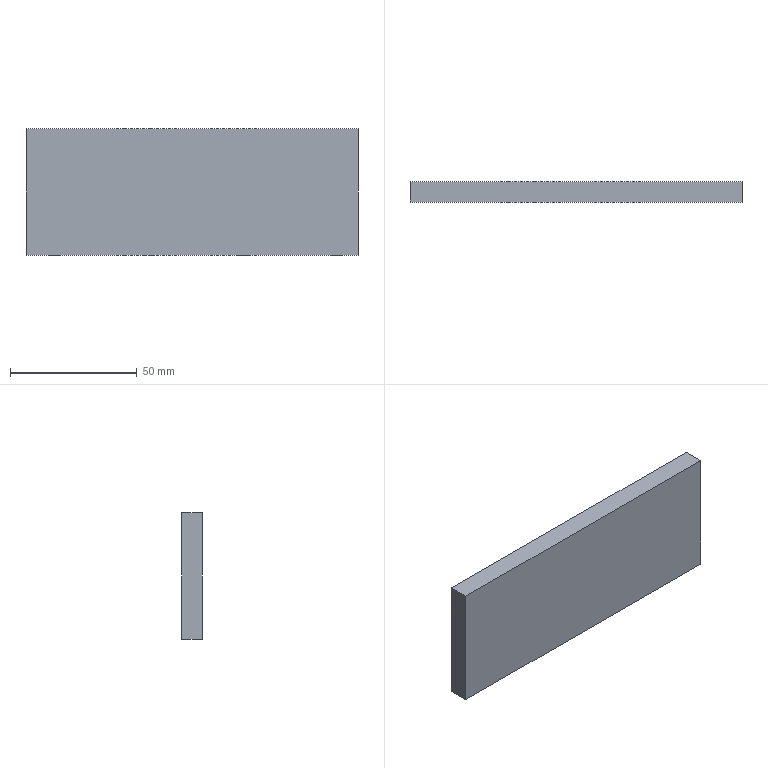Part | SolidWorks | features Extrusion 1, ICE 1 | 1 solid | 18 faces | box 131 x 8 x 50 mm | volume 51646 mm3 | plane 10 | cylinder 8 | commonest cylinder face diameters 4 x8
STEP:
#1=CARTESIAN_POINT('',(124.391,4.,15.));
#2=VERTEX_POINT('',#1);
#3=CARTESIAN_POINT('',(120.391,4.,15.));
#4=VERTEX_POINT('',#3);
#5=CARTESIAN_POINT('',(122.391,4.,15.));
#6=DIRECTION('',(0.,0.,-1.));
#7=DIRECTION('',(-1.,0.,0.));
#8=AXIS2_PLACEMENT_3D('',#5,#6,#7);
#9=CIRCLE('',#8,2.);
#10=EDGE_CURVE('',#2,#4,#9,.T.);
#11=ORIENTED_EDGE('',*,*,#10,.F.);
#12=CARTESIAN_POINT('',(124.391,4.,0.));
#13=VERTEX_POINT('',#12);
#14=CARTESIAN_POINT('',(124.391,4.,15.));
#15=DIRECTION('',(0.,0.,-1.));
#16=VECTOR('',#15,1000.);
#17=LINE('',#14,#16);
#18=EDGE_CURVE('',#2,#13,#17,.T.);
#19=ORIENTED_EDGE('',*,*,#18,.T.);
#20=CARTESIAN_POINT('',(120.391,4.,0.));
#21=VERTEX_POINT('',#20);
#22=CARTESIAN_POINT('',(122.391,4.,0.));
#23=DIRECTION('',(0.,0.,-1.));
#24=DIRECTION('',(-1.,0.,0.));
#25=AXIS2_PLACEMENT_3D('',#22,#23,#24);
#26=CIRCLE('',#25,2.);
#27=EDGE_CURVE('',#13,#21,#26,.T.);
#28=ORIENTED_EDGE('',*,*,#27,.T.);
#29=CARTESIAN_POINT('',(120.391,4.,15.));
#30=DIRECTION('',(0.,0.,-1.));
#31=VECTOR('',#30,1000.);
#32=LINE('',#29,#31);
#33=EDGE_CURVE('',#4,#21,#32,.T.);
#34=ORIENTED_EDGE('',*,*,#33,.F.);
#35=EDGE_LOOP('',(#11,#19,#28,#34));
#36=FACE_OUTER_BOUND('',#35,.T.);
#37=CARTESIAN_POINT('',(122.391,4.,15.));
#38=DIRECTION('',(0.,0.,-1.));
#39=DIRECTION('',(-1.,0.,0.));
#40=AXIS2_PLACEMENT_3D('',#37,#38,#39);
#41=CYLINDRICAL_SURFACE('',#40,2.);
#42=ADVANCED_FACE('',(#36),#41,.F.);
#43=CARTESIAN_POINT('',(87.391,4.,15.));
#44=VERTEX_POINT('',#43);
#45=CARTESIAN_POINT('',(83.391,4.,15.));
#46=VERTEX_POINT('',#45);
#47=CARTESIAN_POINT('',(85.391,4.,15.));
#48=DIRECTION('',(0.,0.,-1.));
#49=DIRECTION('',(-1.,0.,0.));
#50=AXIS2_PLACEMENT_3D('',#47,#48,#49);
#51=CIRCLE('',#50,2.);
#52=EDGE_CURVE('',#44,#46,#51,.T.);
#53=ORIENTED_EDGE('',*,*,#52,.F.);
#54=CARTESIAN_POINT('',(87.391,4.,0.));
#55=VERTEX_POINT('',#54);
#56=CARTESIAN_POINT('',(87.391,4.,15.));
#57=DIRECTION('',(0.,0.,-1.));
#58=VECTOR('',#57,1000.);
#59=LINE('',#56,#58);
#60=EDGE_CURVE('',#44,#55,#59,.T.);
#61=ORIENTED_EDGE('',*,*,#60,.T.);
#62=CARTESIAN_POINT('',(83.391,4.,0.));
#63=VERTEX_POINT('',#62);
#64=CARTESIAN_POINT('',(85.391,4.,0.));
#65=DIRECTION('',(0.,0.,-1.));
#66=DIRECTION('',(-1.,0.,0.));
#67=AXIS2_PLACEMENT_3D('',#64,#65,#66);
#68=CIRCLE('',#67,2.);
#69=EDGE_CURVE('',#55,#63,#68,.T.);
#70=ORIENTED_EDGE('',*,*,#69,.T.);
#71=CARTESIAN_POINT('',(83.391,4.,15.));
#72=DIRECTION('',(0.,0.,-1.));
#73=VECTOR('',#72,1000.);
#74=LINE('',#71,#73);
#75=EDGE_CURVE('',#46,#63,#74,.T.);
#76=ORIENTED_EDGE('',*,*,#75,.F.);
#77=EDGE_LOOP('',(#53,#61,#70,#76));
#78=FACE_OUTER_BOUND('',#77,.T.);
#79=CARTESIAN_POINT('',(85.391,4.,15.));
#80=DIRECTION('',(0.,0.,-1.));
#81=DIRECTION('',(-1.,0.,0.));
#82=AXIS2_PLACEMENT_3D('',#79,#80,#81);
#83=CYLINDRICAL_SURFACE('',#82,2.);
#84=ADVANCED_FACE('',(#78),#83,.F.);
#85=CARTESIAN_POINT('',(50.391,4.,15.));
#86=VERTEX_POINT('',#85);
#87=CARTESIAN_POINT('',(46.391,4.,15.));
#88=VERTEX_POINT('',#87);
#89=CARTESIAN_POINT('',(48.391,4.,15.));
#90=DIRECTION('',(0.,0.,-1.));
#91=DIRECTION('',(-1.,0.,0.));
#92=AXIS2_PLACEMENT_3D('',#89,#90,#91);
#93=CIRCLE('',#92,2.);
#94=EDGE_CURVE('',#86,#88,#93,.T.);
#95=ORIENTED_EDGE('',*,*,#94,.F.);
#96=CARTESIAN_POINT('',(50.391,4.,0.));
#97=VERTEX_POINT('',#96);
#98=CARTESIAN_POINT('',(50.391,4.,15.));
#99=DIRECTION('',(0.,0.,-1.));
#100=VECTOR('',#99,1000.);
#101=LINE('',#98,#100);
#102=EDGE_CURVE('',#86,#97,#101,.T.);
#103=ORIENTED_EDGE('',*,*,#102,.T.);
#104=CARTESIAN_POINT('',(46.391,4.,0.));
#105=VERTEX_POINT('',#104);
#106=CARTESIAN_POINT('',(48.391,4.,0.));
#107=DIRECTION('',(0.,0.,-1.));
#108=DIRECTION('',(-1.,0.,0.));
#109=AXIS2_PLACEMENT_3D('',#106,#107,#108);
#110=CIRCLE('',#109,2.);
#111=EDGE_CURVE('',#97,#105,#110,.T.);
#112=ORIENTED_EDGE('',*,*,#111,.T.);
#113=CARTESIAN_POINT('',(46.391,4.,15.));
#114=DIRECTION('',(0.,0.,-1.));
#115=VECTOR('',#114,1000.);
#116=LINE('',#113,#115);
#117=EDGE_CURVE('',#88,#105,#116,.T.);
#118=ORIENTED_EDGE('',*,*,#117,.F.);
#119=EDGE_LOOP('',(#95,#103,#112,#118));
#120=FACE_OUTER_BOUND('',#119,.T.);
#121=CARTESIAN_POINT('',(48.391,4.,15.));
#122=DIRECTION('',(0.,0.,-1.));
#123=DIRECTION('',(-1.,0.,0.));
#124=AXIS2_PLACEMENT_3D('',#121,#122,#123);
#125=CYLINDRICAL_SURFACE('',#124,2.);
#126=ADVANCED_FACE('',(#120),#125,.F.);
#127=CARTESIAN_POINT('',(13.391,4.,15.));
#128=VERTEX_POINT('',#127);
#129=CARTESIAN_POINT('',(9.391,4.,15.));
#130=VERTEX_POINT('',#129);
#131=CARTESIAN_POINT('',(11.391,4.,15.));
#132=DIRECTION('',(0.,0.,-1.));
#133=DIRECTION('',(-1.,0.,0.));
#134=AXIS2_PLACEMENT_3D('',#131,#132,#133);
#135=CIRCLE('',#134,2.);
#136=EDGE_CURVE('',#128,#130,#135,.T.);
#137=ORIENTED_EDGE('',*,*,#136,.F.);
#138=CARTESIAN_POINT('',(13.391,4.,0.));
#139=VERTEX_POINT('',#138);
#140=CARTESIAN_POINT('',(13.391,4.,15.));
#141=DIRECTION('',(0.,0.,-1.));
#142=VECTOR('',#141,1000.);
#143=LINE('',#140,#142);
#144=EDGE_CURVE('',#128,#139,#143,.T.);
#145=ORIENTED_EDGE('',*,*,#144,.T.);
#146=CARTESIAN_POINT('',(9.391,4.,0.));
#147=VERTEX_POINT('',#146);
#148=CARTESIAN_POINT('',(11.391,4.,0.));
#149=DIRECTION('',(0.,0.,-1.));
#150=DIRECTION('',(-1.,0.,0.));
#151=AXIS2_PLACEMENT_3D('',#148,#149,#150);
#152=CIRCLE('',#151,2.);
#153=EDGE_CURVE('',#139,#147,#152,.T.);
#154=ORIENTED_EDGE('',*,*,#153,.T.);
#155=CARTESIAN_POINT('',(9.391,4.,15.));
#156=DIRECTION('',(0.,0.,-1.));
#157=VECTOR('',#156,1000.);
#158=LINE('',#155,#157);
#159=EDGE_CURVE('',#130,#147,#158,.T.);
#160=ORIENTED_EDGE('',*,*,#159,.F.);
#161=EDGE_LOOP('',(#137,#145,#154,#160));
#162=FACE_OUTER_BOUND('',#161,.T.);
#163=CARTESIAN_POINT('',(11.391,4.,15.));
#164=DIRECTION('',(0.,0.,-1.));
#165=DIRECTION('',(-1.,0.,0.));
#166=AXIS2_PLACEMENT_3D('',#163,#164,#165);
#167=CYLINDRICAL_SURFACE('',#166,2.);
#168=ADVANCED_FACE('',(#162),#167,.F.);
#169=CARTESIAN_POINT('',(0.,8.,0.));
#170=VERTEX_POINT('',#169);
#171=CARTESIAN_POINT('',(0.,0.,0.));
#172=VERTEX_POINT('',#171);
#173=CARTESIAN_POINT('',(0.,0.,0.));
#174=DIRECTION('',(0.,-1.,0.));
#175=VECTOR('',#174,1000.);
#176=LINE('',#173,#175);
#177=EDGE_CURVE('',#170,#172,#176,.T.);
#178=ORIENTED_EDGE('',*,*,#177,.T.);
#179=CARTESIAN_POINT('',(0.,0.,50.));
#180=VERTEX_POINT('',#179);
#181=CARTESIAN_POINT('',(0.,0.,50.));
#182=DIRECTION('',(0.,0.,-1.));
#183=VECTOR('',#182,1000.);
#184=LINE('',#181,#183);
#185=EDGE_CURVE('',#180,#172,#184,.T.);
#186=ORIENTED_EDGE('',*,*,#185,.F.);
#187=CARTESIAN_POINT('',(0.,8.,50.));
#188=VERTEX_POINT('',#187);
#189=CARTESIAN_POINT('',(0.,0.,50.));
#190=DIRECTION('',(0.,-1.,0.));
#191=VECTOR('',#190,1000.);
#192=LINE('',#189,#191);
#193=EDGE_CURVE('',#188,#180,#192,.T.);
#194=ORIENTED_EDGE('',*,*,#193,.F.);
#195=CARTESIAN_POINT('',(0.,8.,50.));
#196=DIRECTION('',(0.,0.,-1.));
#197=VECTOR('',#196,1000.);
#198=LINE('',#195,#197);
#199=EDGE_CURVE('',#188,#170,#198,.T.);
#200=ORIENTED_EDGE('',*,*,#199,.T.);
#201=EDGE_LOOP('',(#178,#186,#194,#200));
#202=FACE_OUTER_BOUND('',#201,.T.);
#203=CARTESIAN_POINT('',(0.,0.,50.));
#204=DIRECTION('',(1.,0.,0.));
#205=DIRECTION('',(0.,0.,-1.));
#206=AXIS2_PLACEMENT_3D('',#203,#204,#205);
#207=PLANE('',#206);
#208=ADVANCED_FACE('',(#202),#207,.F.);
#209=CARTESIAN_POINT('',(131.,0.,0.));
#210=VERTEX_POINT('',#209);
#211=CARTESIAN_POINT('',(0.,0.,0.));
#212=DIRECTION('',(1.,0.,0.));
#213=VECTOR('',#212,1000.);
#214=LINE('',#211,#213);
#215=EDGE_CURVE('',#172,#210,#214,.T.);
#216=ORIENTED_EDGE('',*,*,#215,.T.);
#217=CARTESIAN_POINT('',(131.,0.,50.));
#218=VERTEX_POINT('',#217);
#219=CARTESIAN_POINT('',(131.,0.,50.));
#220=DIRECTION('',(0.,0.,-1.));
#221=VECTOR('',#220,1000.);
#222=LINE('',#219,#221);
#223=EDGE_CURVE('',#218,#210,#222,.T.);
#224=ORIENTED_EDGE('',*,*,#223,.F.);
#225=CARTESIAN_POINT('',(0.,0.,50.));
#226=DIRECTION('',(1.,0.,0.));
#227=VECTOR('',#226,1000.);
#228=LINE('',#225,#227);
#229=EDGE_CURVE('',#180,#218,#228,.T.);
#230=ORIENTED_EDGE('',*,*,#229,.F.);
#231=ORIENTED_EDGE('',*,*,#185,.T.);
#232=EDGE_LOOP('',(#216,#224,#230,#231));
#233=FACE_OUTER_BOUND('',#232,.T.);
#234=CARTESIAN_POINT('',(0.,0.,50.));
#235=DIRECTION('',(0.,1.,0.));
#236=DIRECTION('',(0.,0.,1.));
#237=AXIS2_PLACEMENT_3D('',#234,#235,#236);
#238=PLANE('',#237);
#239=ADVANCED_FACE('',(#233),#238,.F.);
#240=CARTESIAN_POINT('',(131.,8.,0.));
#241=VERTEX_POINT('',#240);
#242=CARTESIAN_POINT('',(131.,0.,0.));
#243=DIRECTION('',(0.,1.,0.));
#244=VECTOR('',#243,1000.);
#245=LINE('',#242,#244);
#246=EDGE_CURVE('',#210,#241,#245,.T.);
#247=ORIENTED_EDGE('',*,*,#246,.T.);
#248=CARTESIAN_POINT('',(131.,8.,50.));
#249=VERTEX_POINT('',#248);
#250=CARTESIAN_POINT('',(131.,8.,50.));
#251=DIRECTION('',(0.,0.,-1.));
#252=VECTOR('',#251,1000.);
#253=LINE('',#250,#252);
#254=EDGE_CURVE('',#249,#241,#253,.T.);
#255=ORIENTED_EDGE('',*,*,#254,.F.);
#256=CARTESIAN_POINT('',(131.,0.,50.));
#257=DIRECTION('',(0.,1.,0.));
#258=VECTOR('',#257,1000.);
#259=LINE('',#256,#258);
#260=EDGE_CURVE('',#218,#249,#259,.T.);
#261=ORIENTED_EDGE('',*,*,#260,.F.);
#262=ORIENTED_EDGE('',*,*,#223,.T.);
#263=EDGE_LOOP('',(#247,#255,#261,#262));
#264=FACE_OUTER_BOUND('',#263,.T.);
#265=CARTESIAN_POINT('',(131.,0.,50.));
#266=DIRECTION('',(-1.,0.,0.));
#267=DIRECTION('',(0.,0.,1.));
#268=AXIS2_PLACEMENT_3D('',#265,#266,#267);
#269=PLANE('',#268);
#270=ADVANCED_FACE('',(#264),#269,.F.);
#271=CARTESIAN_POINT('',(0.,8.,0.));
#272=DIRECTION('',(-1.,0.,0.));
#273=VECTOR('',#272,1000.);
#274=LINE('',#271,#273);
#275=EDGE_CURVE('',#241,#170,#274,.T.);
#276=ORIENTED_EDGE('',*,*,#275,.T.);
#277=ORIENTED_EDGE('',*,*,#199,.F.);
#278=CARTESIAN_POINT('',(0.,8.,50.));
#279=DIRECTION('',(-1.,0.,0.));
#280=VECTOR('',#279,1000.);
#281=LINE('',#278,#280);
#282=EDGE_CURVE('',#249,#188,#281,.T.);
#283=ORIENTED_EDGE('',*,*,#282,.F.);
#284=ORIENTED_EDGE('',*,*,#254,.T.);
#285=EDGE_LOOP('',(#276,#277,#283,#284));
#286=FACE_OUTER_BOUND('',#285,.T.);
#287=CARTESIAN_POINT('',(0.,8.,50.));
#288=DIRECTION('',(0.,-1.,0.));
#289=DIRECTION('',(0.,0.,-1.));
#290=AXIS2_PLACEMENT_3D('',#287,#288,#289);
#291=PLANE('',#290);
#292=ADVANCED_FACE('',(#286),#291,.F.);
#293=ORIENTED_EDGE('',*,*,#193,.T.);
#294=ORIENTED_EDGE('',*,*,#229,.T.);
#295=ORIENTED_EDGE('',*,*,#260,.T.);
#296=ORIENTED_EDGE('',*,*,#282,.T.);
#297=EDGE_LOOP('',(#293,#294,#295,#296));
#298=FACE_OUTER_BOUND('',#297,.T.);
#299=CARTESIAN_POINT('',(0.,0.,50.));
#300=DIRECTION('',(0.,0.,-1.));
#301=DIRECTION('',(-1.,0.,0.));
#302=AXIS2_PLACEMENT_3D('',#299,#300,#301);
#303=PLANE('',#302);
#304=ADVANCED_FACE('',(#298),#303,.F.);
#305=CARTESIAN_POINT('',(122.391,4.,0.));
#306=DIRECTION('',(0.,0.,-1.));
#307=DIRECTION('',(-1.,0.,0.));
#308=AXIS2_PLACEMENT_3D('',#305,#306,#307);
#309=CIRCLE('',#308,2.);
#310=EDGE_CURVE('',#21,#13,#309,.T.);
#311=ORIENTED_EDGE('',*,*,#310,.F.);
#312=ORIENTED_EDGE('',*,*,#27,.F.);
#313=EDGE_LOOP('',(#311,#312));
#314=FACE_BOUND('',#313,.T.);
#315=CARTESIAN_POINT('',(85.391,4.,0.));
#316=DIRECTION('',(0.,0.,-1.));
#317=DIRECTION('',(-1.,0.,0.));
#318=AXIS2_PLACEMENT_3D('',#315,#316,#317);
#319=CIRCLE('',#318,2.);
#320=EDGE_CURVE('',#63,#55,#319,.T.);
#321=ORIENTED_EDGE('',*,*,#320,.F.);
#322=ORIENTED_EDGE('',*,*,#69,.F.);
#323=EDGE_LOOP('',(#321,#322));
#324=FACE_BOUND('',#323,.T.);
#325=CARTESIAN_POINT('',(48.391,4.,0.));
#326=DIRECTION('',(0.,0.,-1.));
#327=DIRECTION('',(-1.,0.,0.));
#328=AXIS2_PLACEMENT_3D('',#325,#326,#327);
#329=CIRCLE('',#328,2.);
#330=EDGE_CURVE('',#105,#97,#329,.T.);
#331=ORIENTED_EDGE('',*,*,#330,.F.);
#332=ORIENTED_EDGE('',*,*,#111,.F.);
#333=EDGE_LOOP('',(#331,#332));
#334=FACE_BOUND('',#333,.T.);
#335=CARTESIAN_POINT('',(11.391,4.,0.));
#336=DIRECTION('',(0.,0.,-1.));
#337=DIRECTION('',(-1.,0.,0.));
#338=AXIS2_PLACEMENT_3D('',#335,#336,#337);
#339=CIRCLE('',#338,2.);
#340=EDGE_CURVE('',#147,#139,#339,.T.);
#341=ORIENTED_EDGE('',*,*,#340,.F.);
#342=ORIENTED_EDGE('',*,*,#153,.F.);
#343=EDGE_LOOP('',(#341,#342));
#344=FACE_BOUND('',#343,.T.);
#345=ORIENTED_EDGE('',*,*,#177,.F.);
#346=ORIENTED_EDGE('',*,*,#275,.F.);
#347=ORIENTED_EDGE('',*,*,#246,.F.);
#348=ORIENTED_EDGE('',*,*,#215,.F.);
#349=EDGE_LOOP('',(#345,#346,#347,#348));
#350=FACE_OUTER_BOUND('',#349,.T.);
#351=CARTESIAN_POINT('',(0.,0.,0.));
#352=DIRECTION('',(0.,0.,-1.));
#353=DIRECTION('',(-1.,0.,0.));
#354=AXIS2_PLACEMENT_3D('',#351,#352,#353);
#355=PLANE('',#354);
#356=ADVANCED_FACE('',(#314,#324,#334,#344,#350),#355,.T.);
#357=ORIENTED_EDGE('',*,*,#144,.F.);
#358=CARTESIAN_POINT('',(11.391,4.,15.));
#359=DIRECTION('',(0.,0.,-1.));
#360=DIRECTION('',(-1.,0.,0.));
#361=AXIS2_PLACEMENT_3D('',#358,#359,#360);
#362=CIRCLE('',#361,2.);
#363=EDGE_CURVE('',#130,#128,#362,.T.);
#364=ORIENTED_EDGE('',*,*,#363,.F.);
#365=ORIENTED_EDGE('',*,*,#159,.T.);
#366=ORIENTED_EDGE('',*,*,#340,.T.);
#367=EDGE_LOOP('',(#357,#364,#365,#366));
#368=FACE_OUTER_BOUND('',#367,.T.);
#369=CARTESIAN_POINT('',(11.391,4.,15.));
#370=DIRECTION('',(0.,0.,-1.));
#371=DIRECTION('',(-1.,0.,0.));
#372=AXIS2_PLACEMENT_3D('',#369,#370,#371);
#373=CYLINDRICAL_SURFACE('',#372,2.);
#374=ADVANCED_FACE('',(#368),#373,.F.);
#375=ORIENTED_EDGE('',*,*,#363,.T.);
#376=ORIENTED_EDGE('',*,*,#136,.T.);
#377=EDGE_LOOP('',(#375,#376));
#378=FACE_OUTER_BOUND('',#377,.T.);
#379=CARTESIAN_POINT('',(11.391,4.,15.));
#380=DIRECTION('',(0.,0.,-1.));
#381=DIRECTION('',(-1.,0.,0.));
#382=AXIS2_PLACEMENT_3D('',#379,#380,#381);
#383=PLANE('',#382);
#384=ADVANCED_FACE('',(#378),#383,.T.);
#385=ORIENTED_EDGE('',*,*,#102,.F.);
#386=CARTESIAN_POINT('',(48.391,4.,15.));
#387=DIRECTION('',(0.,0.,-1.));
#388=DIRECTION('',(-1.,0.,0.));
#389=AXIS2_PLACEMENT_3D('',#386,#387,#388);
#390=CIRCLE('',#389,2.);
#391=EDGE_CURVE('',#88,#86,#390,.T.);
#392=ORIENTED_EDGE('',*,*,#391,.F.);
#393=ORIENTED_EDGE('',*,*,#117,.T.);
#394=ORIENTED_EDGE('',*,*,#330,.T.);
#395=EDGE_LOOP('',(#385,#392,#393,#394));
#396=FACE_OUTER_BOUND('',#395,.T.);
#397=CARTESIAN_POINT('',(48.391,4.,15.));
#398=DIRECTION('',(0.,0.,-1.));
#399=DIRECTION('',(-1.,0.,0.));
#400=AXIS2_PLACEMENT_3D('',#397,#398,#399);
#401=CYLINDRICAL_SURFACE('',#400,2.);
#402=ADVANCED_FACE('',(#396),#401,.F.);
#403=ORIENTED_EDGE('',*,*,#391,.T.);
#404=ORIENTED_EDGE('',*,*,#94,.T.);
#405=EDGE_LOOP('',(#403,#404));
#406=FACE_OUTER_BOUND('',#405,.T.);
#407=CARTESIAN_POINT('',(48.391,4.,15.));
#408=DIRECTION('',(0.,0.,-1.));
#409=DIRECTION('',(-1.,0.,0.));
#410=AXIS2_PLACEMENT_3D('',#407,#408,#409);
#411=PLANE('',#410);
#412=ADVANCED_FACE('',(#406),#411,.T.);
#413=ORIENTED_EDGE('',*,*,#60,.F.);
#414=CARTESIAN_POINT('',(85.391,4.,15.));
#415=DIRECTION('',(0.,0.,-1.));
#416=DIRECTION('',(-1.,0.,0.));
#417=AXIS2_PLACEMENT_3D('',#414,#415,#416);
#418=CIRCLE('',#417,2.);
#419=EDGE_CURVE('',#46,#44,#418,.T.);
#420=ORIENTED_EDGE('',*,*,#419,.F.);
#421=ORIENTED_EDGE('',*,*,#75,.T.);
#422=ORIENTED_EDGE('',*,*,#320,.T.);
#423=EDGE_LOOP('',(#413,#420,#421,#422));
#424=FACE_OUTER_BOUND('',#423,.T.);
#425=CARTESIAN_POINT('',(85.391,4.,15.));
#426=DIRECTION('',(0.,0.,-1.));
#427=DIRECTION('',(-1.,0.,0.));
#428=AXIS2_PLACEMENT_3D('',#425,#426,#427);
#429=CYLINDRICAL_SURFACE('',#428,2.);
#430=ADVANCED_FACE('',(#424),#429,.F.);
#431=ORIENTED_EDGE('',*,*,#419,.T.);
#432=ORIENTED_EDGE('',*,*,#52,.T.);
#433=EDGE_LOOP('',(#431,#432));
#434=FACE_OUTER_BOUND('',#433,.T.);
#435=CARTESIAN_POINT('',(85.391,4.,15.));
#436=DIRECTION('',(0.,0.,-1.));
#437=DIRECTION('',(-1.,0.,0.));
#438=AXIS2_PLACEMENT_3D('',#435,#436,#437);
#439=PLANE('',#438);
#440=ADVANCED_FACE('',(#434),#439,.T.);
#441=ORIENTED_EDGE('',*,*,#18,.F.);
#442=CARTESIAN_POINT('',(122.391,4.,15.));
#443=DIRECTION('',(0.,0.,-1.));
#444=DIRECTION('',(-1.,0.,0.));
#445=AXIS2_PLACEMENT_3D('',#442,#443,#444);
#446=CIRCLE('',#445,2.);
#447=EDGE_CURVE('',#4,#2,#446,.T.);
#448=ORIENTED_EDGE('',*,*,#447,.F.);
#449=ORIENTED_EDGE('',*,*,#33,.T.);
#450=ORIENTED_EDGE('',*,*,#310,.T.);
#451=EDGE_LOOP('',(#441,#448,#449,#450));
#452=FACE_OUTER_BOUND('',#451,.T.);
#453=CARTESIAN_POINT('',(122.391,4.,15.));
#454=DIRECTION('',(0.,0.,-1.));
#455=DIRECTION('',(-1.,0.,0.));
#456=AXIS2_PLACEMENT_3D('',#453,#454,#455);
#457=CYLINDRICAL_SURFACE('',#456,2.);
#458=ADVANCED_FACE('',(#452),#457,.F.);
#459=ORIENTED_EDGE('',*,*,#447,.T.);
#460=ORIENTED_EDGE('',*,*,#10,.T.);
#461=EDGE_LOOP('',(#459,#460));
#462=FACE_OUTER_BOUND('',#461,.T.);
#463=CARTESIAN_POINT('',(122.391,4.,15.));
#464=DIRECTION('',(0.,0.,-1.));
#465=DIRECTION('',(-1.,0.,0.));
#466=AXIS2_PLACEMENT_3D('',#463,#464,#465);
#467=PLANE('',#466);
#468=ADVANCED_FACE('',(#462),#467,.T.);
#469=CLOSED_SHELL('',(#42,#84,#126,#168,#208,#239,#270,#292,#304,#356,#374,#384,#402,#412,#430,#440,#458,#468));
#470=MANIFOLD_SOLID_BREP('',#469);
#471=CARTESIAN_POINT('',(0.,0.,0.));
#472=DIRECTION('',(0.,0.,1.));
#473=DIRECTION('',(1.,0.,0.));
#474=AXIS2_PLACEMENT_3D('',#471,#472,#473);
#475=(LENGTH_UNIT()NAMED_UNIT(*)SI_UNIT(.MILLI.,.METRE.));
#476=UNCERTAINTY_MEASURE_WITH_UNIT(LENGTH_MEASURE(0.00001),#475,'','');
#477=(NAMED_UNIT(*)PLANE_ANGLE_UNIT()SI_UNIT($,.RADIAN.));
#478=(NAMED_UNIT(*)SI_UNIT($,.STERADIAN.)SOLID_ANGLE_UNIT());
#479=(GEOMETRIC_REPRESENTATION_CONTEXT(3)GLOBAL_UNCERTAINTY_ASSIGNED_CONTEXT((#476))GLOBAL_UNIT_ASSIGNED_CONTEXT((#475,#477,#478))REPRESENTATION_CONTEXT('',''));
#480=ADVANCED_BREP_SHAPE_REPRESENTATION('',(#470,#474),#479);